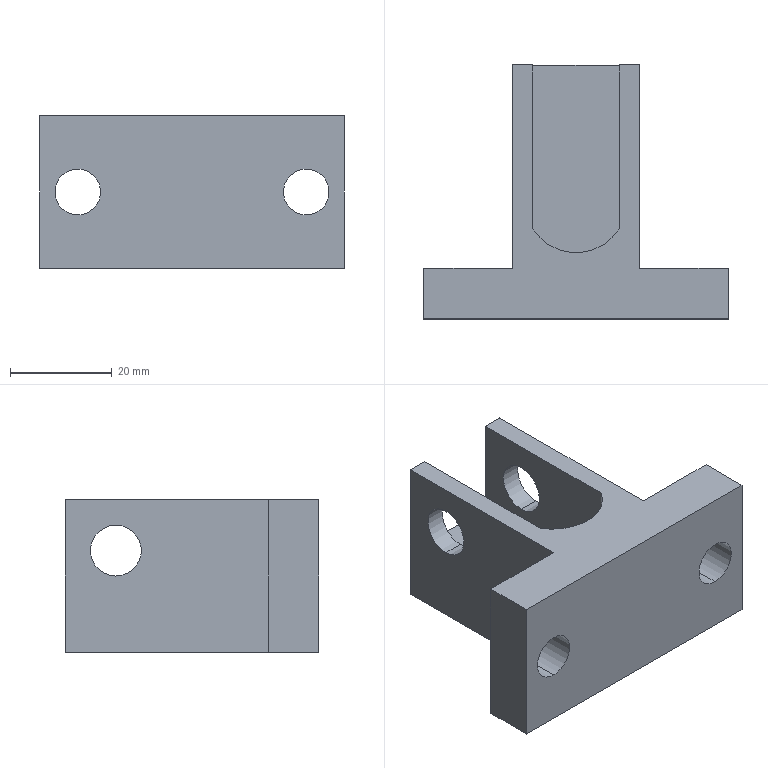Part | SolidWorks | features BaseBody 1 | 1 solid | 22 faces | box 60 x 50 x 30 mm | volume 33992 mm3 | plane 13 | cylinder 9 | commonest cylinder face diameters 9 x4 10 x4 20 x1
STEP:
#1=CARTESIAN_POINT('',(52.5,10.,19.5));
#2=VERTEX_POINT('',#1);
#3=CARTESIAN_POINT('',(52.5,10.,10.5));
#4=VERTEX_POINT('',#3);
#5=CARTESIAN_POINT('',(52.5,10.,15.));
#6=DIRECTION('',(0.,-1.,0.));
#7=DIRECTION('',(0.,0.,-1.));
#8=AXIS2_PLACEMENT_3D('',#5,#6,#7);
#9=CIRCLE('',#8,4.5);
#10=EDGE_CURVE('',#2,#4,#9,.T.);
#11=ORIENTED_EDGE('',*,*,#10,.F.);
#12=CARTESIAN_POINT('',(52.5,0.,19.5));
#13=VERTEX_POINT('',#12);
#14=CARTESIAN_POINT('',(52.5,0.,19.5));
#15=DIRECTION('',(0.,-1.,0.));
#16=VECTOR('',#15,1000.);
#17=LINE('',#14,#16);
#18=EDGE_CURVE('',#2,#13,#17,.T.);
#19=ORIENTED_EDGE('',*,*,#18,.T.);
#20=CARTESIAN_POINT('',(52.5,0.,10.5));
#21=VERTEX_POINT('',#20);
#22=CARTESIAN_POINT('',(52.5,0.,15.));
#23=DIRECTION('',(0.,-1.,0.));
#24=DIRECTION('',(0.,0.,-1.));
#25=AXIS2_PLACEMENT_3D('',#22,#23,#24);
#26=CIRCLE('',#25,4.5);
#27=EDGE_CURVE('',#13,#21,#26,.T.);
#28=ORIENTED_EDGE('',*,*,#27,.T.);
#29=CARTESIAN_POINT('',(52.5,0.,10.5));
#30=DIRECTION('',(0.,-1.,0.));
#31=VECTOR('',#30,1000.);
#32=LINE('',#29,#31);
#33=EDGE_CURVE('',#4,#21,#32,.T.);
#34=ORIENTED_EDGE('',*,*,#33,.F.);
#35=EDGE_LOOP('',(#11,#19,#28,#34));
#36=FACE_OUTER_BOUND('',#35,.T.);
#37=CARTESIAN_POINT('',(52.5,0.,15.));
#38=DIRECTION('',(0.,-1.,0.));
#39=DIRECTION('',(0.,0.,-1.));
#40=AXIS2_PLACEMENT_3D('',#37,#38,#39);
#41=CYLINDRICAL_SURFACE('',#40,4.5);
#42=ADVANCED_FACE('',(#36),#41,.F.);
#43=CARTESIAN_POINT('',(7.5,10.,19.5));
#44=VERTEX_POINT('',#43);
#45=CARTESIAN_POINT('',(7.5,10.,10.5));
#46=VERTEX_POINT('',#45);
#47=CARTESIAN_POINT('',(7.5,10.,15.));
#48=DIRECTION('',(0.,-1.,0.));
#49=DIRECTION('',(0.,0.,-1.));
#50=AXIS2_PLACEMENT_3D('',#47,#48,#49);
#51=CIRCLE('',#50,4.5);
#52=EDGE_CURVE('',#44,#46,#51,.T.);
#53=ORIENTED_EDGE('',*,*,#52,.F.);
#54=CARTESIAN_POINT('',(7.5,0.,19.5));
#55=VERTEX_POINT('',#54);
#56=CARTESIAN_POINT('',(7.5,0.,19.5));
#57=DIRECTION('',(0.,-1.,0.));
#58=VECTOR('',#57,1000.);
#59=LINE('',#56,#58);
#60=EDGE_CURVE('',#44,#55,#59,.T.);
#61=ORIENTED_EDGE('',*,*,#60,.T.);
#62=CARTESIAN_POINT('',(7.5,0.,10.5));
#63=VERTEX_POINT('',#62);
#64=CARTESIAN_POINT('',(7.5,0.,15.));
#65=DIRECTION('',(0.,-1.,0.));
#66=DIRECTION('',(0.,0.,-1.));
#67=AXIS2_PLACEMENT_3D('',#64,#65,#66);
#68=CIRCLE('',#67,4.5);
#69=EDGE_CURVE('',#55,#63,#68,.T.);
#70=ORIENTED_EDGE('',*,*,#69,.T.);
#71=CARTESIAN_POINT('',(7.5,0.,10.5));
#72=DIRECTION('',(0.,-1.,0.));
#73=VECTOR('',#72,1000.);
#74=LINE('',#71,#73);
#75=EDGE_CURVE('',#46,#63,#74,.T.);
#76=ORIENTED_EDGE('',*,*,#75,.F.);
#77=EDGE_LOOP('',(#53,#61,#70,#76));
#78=FACE_OUTER_BOUND('',#77,.T.);
#79=CARTESIAN_POINT('',(7.5,0.,15.));
#80=DIRECTION('',(0.,-1.,0.));
#81=DIRECTION('',(0.,0.,-1.));
#82=AXIS2_PLACEMENT_3D('',#79,#80,#81);
#83=CYLINDRICAL_SURFACE('',#82,4.5);
#84=ADVANCED_FACE('',(#78),#83,.F.);
#85=CARTESIAN_POINT('',(42.5,40.,25.));
#86=VERTEX_POINT('',#85);
#87=CARTESIAN_POINT('',(42.5,40.,15.));
#88=VERTEX_POINT('',#87);
#89=CARTESIAN_POINT('',(42.5,40.,20.));
#90=DIRECTION('',(1.,0.,0.));
#91=DIRECTION('',(0.,0.,1.));
#92=AXIS2_PLACEMENT_3D('',#89,#90,#91);
#93=CIRCLE('',#92,5.);
#94=EDGE_CURVE('',#86,#88,#93,.T.);
#95=ORIENTED_EDGE('',*,*,#94,.T.);
#96=CARTESIAN_POINT('',(38.5,40.,15.));
#97=VERTEX_POINT('',#96);
#98=CARTESIAN_POINT('',(60.,40.,15.));
#99=DIRECTION('',(-1.,0.,0.));
#100=VECTOR('',#99,1000.);
#101=LINE('',#98,#100);
#102=EDGE_CURVE('',#88,#97,#101,.T.);
#103=ORIENTED_EDGE('',*,*,#102,.T.);
#104=CARTESIAN_POINT('',(38.5,40.,25.));
#105=VERTEX_POINT('',#104);
#106=CARTESIAN_POINT('',(38.5,40.,20.));
#107=DIRECTION('',(-1.,0.,0.));
#108=DIRECTION('',(0.,0.,1.));
#109=AXIS2_PLACEMENT_3D('',#106,#107,#108);
#110=CIRCLE('',#109,5.);
#111=EDGE_CURVE('',#97,#105,#110,.T.);
#112=ORIENTED_EDGE('',*,*,#111,.T.);
#113=CARTESIAN_POINT('',(60.,40.,25.));
#114=DIRECTION('',(-1.,0.,0.));
#115=VECTOR('',#114,1000.);
#116=LINE('',#113,#115);
#117=EDGE_CURVE('',#86,#105,#116,.T.);
#118=ORIENTED_EDGE('',*,*,#117,.F.);
#119=EDGE_LOOP('',(#95,#103,#112,#118));
#120=FACE_OUTER_BOUND('',#119,.T.);
#121=CARTESIAN_POINT('',(60.,40.,20.));
#122=DIRECTION('',(-1.,0.,0.));
#123=DIRECTION('',(0.,0.,1.));
#124=AXIS2_PLACEMENT_3D('',#121,#122,#123);
#125=CYLINDRICAL_SURFACE('',#124,5.);
#126=ADVANCED_FACE('',(#120),#125,.F.);
#127=CARTESIAN_POINT('',(21.5,40.,25.));
#128=VERTEX_POINT('',#127);
#129=CARTESIAN_POINT('',(21.5,40.,15.));
#130=VERTEX_POINT('',#129);
#131=CARTESIAN_POINT('',(21.5,40.,20.));
#132=DIRECTION('',(1.,0.,0.));
#133=DIRECTION('',(0.,0.,1.));
#134=AXIS2_PLACEMENT_3D('',#131,#132,#133);
#135=CIRCLE('',#134,5.);
#136=EDGE_CURVE('',#128,#130,#135,.T.);
#137=ORIENTED_EDGE('',*,*,#136,.T.);
#138=CARTESIAN_POINT('',(17.5,40.,15.));
#139=VERTEX_POINT('',#138);
#140=CARTESIAN_POINT('',(60.,40.,15.));
#141=DIRECTION('',(-1.,0.,0.));
#142=VECTOR('',#141,1000.);
#143=LINE('',#140,#142);
#144=EDGE_CURVE('',#130,#139,#143,.T.);
#145=ORIENTED_EDGE('',*,*,#144,.T.);
#146=CARTESIAN_POINT('',(17.5,40.,25.));
#147=VERTEX_POINT('',#146);
#148=CARTESIAN_POINT('',(17.5,40.,20.));
#149=DIRECTION('',(-1.,0.,0.));
#150=DIRECTION('',(0.,0.,1.));
#151=AXIS2_PLACEMENT_3D('',#148,#149,#150);
#152=CIRCLE('',#151,5.);
#153=EDGE_CURVE('',#139,#147,#152,.T.);
#154=ORIENTED_EDGE('',*,*,#153,.T.);
#155=CARTESIAN_POINT('',(60.,40.,25.));
#156=DIRECTION('',(-1.,0.,0.));
#157=VECTOR('',#156,1000.);
#158=LINE('',#155,#157);
#159=EDGE_CURVE('',#128,#147,#158,.T.);
#160=ORIENTED_EDGE('',*,*,#159,.F.);
#161=EDGE_LOOP('',(#137,#145,#154,#160));
#162=FACE_OUTER_BOUND('',#161,.T.);
#163=CARTESIAN_POINT('',(60.,40.,20.));
#164=DIRECTION('',(-1.,0.,0.));
#165=DIRECTION('',(0.,0.,1.));
#166=AXIS2_PLACEMENT_3D('',#163,#164,#165);
#167=CYLINDRICAL_SURFACE('',#166,5.);
#168=ADVANCED_FACE('',(#162),#167,.F.);
#169=CARTESIAN_POINT('',(60.,0.,30.));
#170=VERTEX_POINT('',#169);
#171=CARTESIAN_POINT('',(60.,0.,0.));
#172=VERTEX_POINT('',#171);
#173=CARTESIAN_POINT('',(60.,0.,30.));
#174=DIRECTION('',(0.,0.,-1.));
#175=VECTOR('',#174,1000.);
#176=LINE('',#173,#175);
#177=EDGE_CURVE('',#170,#172,#176,.T.);
#178=ORIENTED_EDGE('',*,*,#177,.F.);
#179=CARTESIAN_POINT('',(0.,0.,30.));
#180=VERTEX_POINT('',#179);
#181=CARTESIAN_POINT('',(60.,0.,30.));
#182=DIRECTION('',(1.,0.,0.));
#183=VECTOR('',#182,1000.);
#184=LINE('',#181,#183);
#185=EDGE_CURVE('',#180,#170,#184,.T.);
#186=ORIENTED_EDGE('',*,*,#185,.F.);
#187=CARTESIAN_POINT('',(0.,0.,0.));
#188=VERTEX_POINT('',#187);
#189=CARTESIAN_POINT('',(0.,0.,30.));
#190=DIRECTION('',(0.,0.,1.));
#191=VECTOR('',#190,1000.);
#192=LINE('',#189,#191);
#193=EDGE_CURVE('',#188,#180,#192,.T.);
#194=ORIENTED_EDGE('',*,*,#193,.F.);
#195=CARTESIAN_POINT('',(60.,0.,0.));
#196=DIRECTION('',(-1.,0.,0.));
#197=VECTOR('',#196,1000.);
#198=LINE('',#195,#197);
#199=EDGE_CURVE('',#172,#188,#198,.T.);
#200=ORIENTED_EDGE('',*,*,#199,.F.);
#201=EDGE_LOOP('',(#178,#186,#194,#200));
#202=FACE_OUTER_BOUND('',#201,.T.);
#203=CARTESIAN_POINT('',(52.5,0.,15.));
#204=DIRECTION('',(0.,-1.,0.));
#205=DIRECTION('',(0.,0.,-1.));
#206=AXIS2_PLACEMENT_3D('',#203,#204,#205);
#207=CIRCLE('',#206,4.5);
#208=EDGE_CURVE('',#21,#13,#207,.T.);
#209=ORIENTED_EDGE('',*,*,#208,.F.);
#210=ORIENTED_EDGE('',*,*,#27,.F.);
#211=EDGE_LOOP('',(#209,#210));
#212=FACE_BOUND('',#211,.T.);
#213=CARTESIAN_POINT('',(7.5,0.,15.));
#214=DIRECTION('',(0.,-1.,0.));
#215=DIRECTION('',(0.,0.,-1.));
#216=AXIS2_PLACEMENT_3D('',#213,#214,#215);
#217=CIRCLE('',#216,4.5);
#218=EDGE_CURVE('',#63,#55,#217,.T.);
#219=ORIENTED_EDGE('',*,*,#218,.F.);
#220=ORIENTED_EDGE('',*,*,#69,.F.);
#221=EDGE_LOOP('',(#219,#220));
#222=FACE_BOUND('',#221,.T.);
#223=CARTESIAN_POINT('',(60.,0.,30.));
#224=DIRECTION('',(0.,1.,0.));
#225=DIRECTION('',(-1.,0.,0.));
#226=AXIS2_PLACEMENT_3D('',#223,#224,#225);
#227=PLANE('',#226);
#228=ADVANCED_FACE('',(#202,#212,#222),#227,.F.);
#229=CARTESIAN_POINT('',(42.5,10.,0.));
#230=VERTEX_POINT('',#229);
#231=CARTESIAN_POINT('',(60.,10.,0.));
#232=VERTEX_POINT('',#231);
#233=CARTESIAN_POINT('',(0.,10.,0.));
#234=DIRECTION('',(1.,0.,0.));
#235=VECTOR('',#234,1000.);
#236=LINE('',#233,#235);
#237=EDGE_CURVE('',#230,#232,#236,.T.);
#238=ORIENTED_EDGE('',*,*,#237,.T.);
#239=CARTESIAN_POINT('',(60.,0.,0.));
#240=DIRECTION('',(0.,-1.,0.));
#241=VECTOR('',#240,1000.);
#242=LINE('',#239,#241);
#243=EDGE_CURVE('',#232,#172,#242,.T.);
#244=ORIENTED_EDGE('',*,*,#243,.T.);
#245=ORIENTED_EDGE('',*,*,#199,.T.);
#246=CARTESIAN_POINT('',(0.,10.,0.));
#247=VERTEX_POINT('',#246);
#248=CARTESIAN_POINT('',(0.,0.,0.));
#249=DIRECTION('',(0.,1.,0.));
#250=VECTOR('',#249,1000.);
#251=LINE('',#248,#250);
#252=EDGE_CURVE('',#188,#247,#251,.T.);
#253=ORIENTED_EDGE('',*,*,#252,.T.);
#254=CARTESIAN_POINT('',(17.5,10.,0.));
#255=VERTEX_POINT('',#254);
#256=CARTESIAN_POINT('',(0.,10.,0.));
#257=DIRECTION('',(1.,0.,0.));
#258=VECTOR('',#257,1000.);
#259=LINE('',#256,#258);
#260=EDGE_CURVE('',#247,#255,#259,.T.);
#261=ORIENTED_EDGE('',*,*,#260,.T.);
#262=CARTESIAN_POINT('',(17.5,50.,0.));
#263=VERTEX_POINT('',#262);
#264=CARTESIAN_POINT('',(17.5,0.,0.));
#265=DIRECTION('',(0.,1.,0.));
#266=VECTOR('',#265,1000.);
#267=LINE('',#264,#266);
#268=EDGE_CURVE('',#255,#263,#267,.T.);
#269=ORIENTED_EDGE('',*,*,#268,.T.);
#270=CARTESIAN_POINT('',(42.5,50.,0.));
#271=VERTEX_POINT('',#270);
#272=CARTESIAN_POINT('',(0.,50.,0.));
#273=DIRECTION('',(1.,0.,0.));
#274=VECTOR('',#273,1000.);
#275=LINE('',#272,#274);
#276=EDGE_CURVE('',#263,#271,#275,.T.);
#277=ORIENTED_EDGE('',*,*,#276,.T.);
#278=CARTESIAN_POINT('',(42.5,0.,0.));
#279=DIRECTION('',(0.,-1.,0.));
#280=VECTOR('',#279,1000.);
#281=LINE('',#278,#280);
#282=EDGE_CURVE('',#271,#230,#281,.T.);
#283=ORIENTED_EDGE('',*,*,#282,.T.);
#284=EDGE_LOOP('',(#238,#244,#245,#253,#261,#269,#277,#283));
#285=FACE_OUTER_BOUND('',#284,.T.);
#286=CARTESIAN_POINT('',(0.,0.,0.));
#287=DIRECTION('',(0.,0.,-1.));
#288=DIRECTION('',(-1.,0.,0.));
#289=AXIS2_PLACEMENT_3D('',#286,#287,#288);
#290=PLANE('',#289);
#291=ADVANCED_FACE('',(#285),#290,.T.);
#292=CARTESIAN_POINT('',(60.,10.,30.));
#293=VERTEX_POINT('',#292);
#294=CARTESIAN_POINT('',(60.,10.,30.));
#295=DIRECTION('',(0.,0.,-1.));
#296=VECTOR('',#295,1000.);
#297=LINE('',#294,#296);
#298=EDGE_CURVE('',#293,#232,#297,.T.);
#299=ORIENTED_EDGE('',*,*,#298,.F.);
#300=CARTESIAN_POINT('',(60.,10.,30.));
#301=DIRECTION('',(0.,1.,0.));
#302=VECTOR('',#301,1000.);
#303=LINE('',#300,#302);
#304=EDGE_CURVE('',#170,#293,#303,.T.);
#305=ORIENTED_EDGE('',*,*,#304,.F.);
#306=ORIENTED_EDGE('',*,*,#177,.T.);
#307=ORIENTED_EDGE('',*,*,#243,.F.);
#308=EDGE_LOOP('',(#299,#305,#306,#307));
#309=FACE_OUTER_BOUND('',#308,.T.);
#310=CARTESIAN_POINT('',(60.,10.,30.));
#311=DIRECTION('',(-1.,0.,0.));
#312=DIRECTION('',(0.,0.,1.));
#313=AXIS2_PLACEMENT_3D('',#310,#311,#312);
#314=PLANE('',#313);
#315=ADVANCED_FACE('',(#309),#314,.F.);
#316=CARTESIAN_POINT('',(38.5,17.732,30.));
#317=VERTEX_POINT('',#316);
#318=CARTESIAN_POINT('',(38.5,50.,30.));
#319=VERTEX_POINT('',#318);
#320=CARTESIAN_POINT('',(38.5,0.,30.));
#321=DIRECTION('',(0.,1.,0.));
#322=VECTOR('',#321,1000.);
#323=LINE('',#320,#322);
#324=EDGE_CURVE('',#317,#319,#323,.T.);
#325=ORIENTED_EDGE('',*,*,#324,.F.);
#326=CARTESIAN_POINT('',(21.5,17.732,30.));
#327=VERTEX_POINT('',#326);
#328=CARTESIAN_POINT('',(30.,23.,30.));
#329=DIRECTION('',(0.,0.,1.));
#330=DIRECTION('',(1.,0.,0.));
#331=AXIS2_PLACEMENT_3D('',#328,#329,#330);
#332=CIRCLE('',#331,10.);
#333=EDGE_CURVE('',#327,#317,#332,.T.);
#334=ORIENTED_EDGE('',*,*,#333,.F.);
#335=CARTESIAN_POINT('',(21.5,50.,30.));
#336=VERTEX_POINT('',#335);
#337=CARTESIAN_POINT('',(21.5,0.,30.));
#338=DIRECTION('',(0.,-1.,0.));
#339=VECTOR('',#338,1000.);
#340=LINE('',#337,#339);
#341=EDGE_CURVE('',#336,#327,#340,.T.);
#342=ORIENTED_EDGE('',*,*,#341,.F.);
#343=CARTESIAN_POINT('',(17.5,50.,30.));
#344=VERTEX_POINT('',#343);
#345=CARTESIAN_POINT('',(0.,50.,30.));
#346=DIRECTION('',(1.,0.,0.));
#347=VECTOR('',#346,1000.);
#348=LINE('',#345,#347);
#349=EDGE_CURVE('',#344,#336,#348,.T.);
#350=ORIENTED_EDGE('',*,*,#349,.F.);
#351=CARTESIAN_POINT('',(17.5,10.,30.));
#352=VERTEX_POINT('',#351);
#353=CARTESIAN_POINT('',(17.5,0.,30.));
#354=DIRECTION('',(0.,1.,0.));
#355=VECTOR('',#354,1000.);
#356=LINE('',#353,#355);
#357=EDGE_CURVE('',#352,#344,#356,.T.);
#358=ORIENTED_EDGE('',*,*,#357,.F.);
#359=CARTESIAN_POINT('',(0.,10.,30.));
#360=VERTEX_POINT('',#359);
#361=CARTESIAN_POINT('',(0.,10.,30.));
#362=DIRECTION('',(1.,0.,0.));
#363=VECTOR('',#362,1000.);
#364=LINE('',#361,#363);
#365=EDGE_CURVE('',#360,#352,#364,.T.);
#366=ORIENTED_EDGE('',*,*,#365,.F.);
#367=CARTESIAN_POINT('',(0.,0.,30.));
#368=DIRECTION('',(0.,1.,0.));
#369=VECTOR('',#368,1000.);
#370=LINE('',#367,#369);
#371=EDGE_CURVE('',#180,#360,#370,.T.);
#372=ORIENTED_EDGE('',*,*,#371,.F.);
#373=ORIENTED_EDGE('',*,*,#185,.T.);
#374=ORIENTED_EDGE('',*,*,#304,.T.);
#375=CARTESIAN_POINT('',(42.5,10.,30.));
#376=VERTEX_POINT('',#375);
#377=CARTESIAN_POINT('',(0.,10.,30.));
#378=DIRECTION('',(1.,0.,0.));
#379=VECTOR('',#378,1000.);
#380=LINE('',#377,#379);
#381=EDGE_CURVE('',#376,#293,#380,.T.);
#382=ORIENTED_EDGE('',*,*,#381,.F.);
#383=CARTESIAN_POINT('',(42.5,50.,30.));
#384=VERTEX_POINT('',#383);
#385=CARTESIAN_POINT('',(42.5,0.,30.));
#386=DIRECTION('',(0.,-1.,0.));
#387=VECTOR('',#386,1000.);
#388=LINE('',#385,#387);
#389=EDGE_CURVE('',#384,#376,#388,.T.);
#390=ORIENTED_EDGE('',*,*,#389,.F.);
#391=CARTESIAN_POINT('',(0.,50.,30.));
#392=DIRECTION('',(1.,0.,0.));
#393=VECTOR('',#392,1000.);
#394=LINE('',#391,#393);
#395=EDGE_CURVE('',#319,#384,#394,.T.);
#396=ORIENTED_EDGE('',*,*,#395,.F.);
#397=EDGE_LOOP('',(#325,#334,#342,#350,#358,#366,#372,#373,#374,#382,#390,#396));
#398=FACE_OUTER_BOUND('',#397,.T.);
#399=CARTESIAN_POINT('',(0.,0.,30.));
#400=DIRECTION('',(0.,0.,-1.));
#401=DIRECTION('',(-1.,0.,0.));
#402=AXIS2_PLACEMENT_3D('',#399,#400,#401);
#403=PLANE('',#402);
#404=ADVANCED_FACE('',(#398),#403,.F.);
#405=ORIENTED_EDGE('',*,*,#193,.T.);
#406=ORIENTED_EDGE('',*,*,#371,.T.);
#407=CARTESIAN_POINT('',(0.,10.,30.));
#408=DIRECTION('',(0.,0.,1.));
#409=VECTOR('',#408,1000.);
#410=LINE('',#407,#409);
#411=EDGE_CURVE('',#247,#360,#410,.T.);
#412=ORIENTED_EDGE('',*,*,#411,.F.);
#413=ORIENTED_EDGE('',*,*,#252,.F.);
#414=EDGE_LOOP('',(#405,#406,#412,#413));
#415=FACE_OUTER_BOUND('',#414,.T.);
#416=CARTESIAN_POINT('',(0.,0.,30.));
#417=DIRECTION('',(1.,0.,0.));
#418=DIRECTION('',(0.,0.,-1.));
#419=AXIS2_PLACEMENT_3D('',#416,#417,#418);
#420=PLANE('',#419);
#421=ADVANCED_FACE('',(#415),#420,.F.);
#422=ORIENTED_EDGE('',*,*,#18,.F.);
#423=CARTESIAN_POINT('',(52.5,10.,15.));
#424=DIRECTION('',(0.,-1.,0.));
#425=DIRECTION('',(0.,0.,-1.));
#426=AXIS2_PLACEMENT_3D('',#423,#424,#425);
#427=CIRCLE('',#426,4.5);
#428=EDGE_CURVE('',#4,#2,#427,.T.);
#429=ORIENTED_EDGE('',*,*,#428,.F.);
#430=ORIENTED_EDGE('',*,*,#33,.T.);
#431=ORIENTED_EDGE('',*,*,#208,.T.);
#432=EDGE_LOOP('',(#422,#429,#430,#431));
#433=FACE_OUTER_BOUND('',#432,.T.);
#434=CARTESIAN_POINT('',(52.5,0.,15.));
#435=DIRECTION('',(0.,-1.,0.));
#436=DIRECTION('',(0.,0.,-1.));
#437=AXIS2_PLACEMENT_3D('',#434,#435,#436);
#438=CYLINDRICAL_SURFACE('',#437,4.5);
#439=ADVANCED_FACE('',(#433),#438,.F.);
#440=ORIENTED_EDGE('',*,*,#60,.F.);
#441=CARTESIAN_POINT('',(7.5,10.,15.));
#442=DIRECTION('',(0.,-1.,0.));
#443=DIRECTION('',(0.,0.,-1.));
#444=AXIS2_PLACEMENT_3D('',#441,#442,#443);
#445=CIRCLE('',#444,4.5);
#446=EDGE_CURVE('',#46,#44,#445,.T.);
#447=ORIENTED_EDGE('',*,*,#446,.F.);
#448=ORIENTED_EDGE('',*,*,#75,.T.);
#449=ORIENTED_EDGE('',*,*,#218,.T.);
#450=EDGE_LOOP('',(#440,#447,#448,#449));
#451=FACE_OUTER_BOUND('',#450,.T.);
#452=CARTESIAN_POINT('',(7.5,0.,15.));
#453=DIRECTION('',(0.,-1.,0.));
#454=DIRECTION('',(0.,0.,-1.));
#455=AXIS2_PLACEMENT_3D('',#452,#453,#454);
#456=CYLINDRICAL_SURFACE('',#455,4.5);
#457=ADVANCED_FACE('',(#451),#456,.F.);
#458=CARTESIAN_POINT('',(42.5,10.,30.));
#459=DIRECTION('',(0.,0.,-1.));
#460=VECTOR('',#459,1000.);
#461=LINE('',#458,#460);
#462=EDGE_CURVE('',#376,#230,#461,.T.);
#463=ORIENTED_EDGE('',*,*,#462,.F.);
#464=ORIENTED_EDGE('',*,*,#381,.T.);
#465=ORIENTED_EDGE('',*,*,#298,.T.);
#466=ORIENTED_EDGE('',*,*,#237,.F.);
#467=EDGE_LOOP('',(#463,#464,#465,#466));
#468=FACE_OUTER_BOUND('',#467,.T.);
#469=ORIENTED_EDGE('',*,*,#428,.T.);
#470=ORIENTED_EDGE('',*,*,#10,.T.);
#471=EDGE_LOOP('',(#469,#470));
#472=FACE_BOUND('',#471,.T.);
#473=CARTESIAN_POINT('',(42.5,10.,30.));
#474=DIRECTION('',(0.,-1.,0.));
#475=DIRECTION('',(0.,0.,-1.));
#476=AXIS2_PLACEMENT_3D('',#473,#474,#475);
#477=PLANE('',#476);
#478=ADVANCED_FACE('',(#468,#472),#477,.F.);
#479=CARTESIAN_POINT('',(42.5,50.,30.));
#480=DIRECTION('',(0.,0.,-1.));
#481=VECTOR('',#480,1000.);
#482=LINE('',#479,#481);
#483=EDGE_CURVE('',#384,#271,#482,.T.);
#484=ORIENTED_EDGE('',*,*,#483,.F.);
#485=ORIENTED_EDGE('',*,*,#389,.T.);
#486=ORIENTED_EDGE('',*,*,#462,.T.);
#487=ORIENTED_EDGE('',*,*,#282,.F.);
#488=EDGE_LOOP('',(#484,#485,#486,#487));
#489=FACE_OUTER_BOUND('',#488,.T.);
#490=ORIENTED_EDGE('',*,*,#94,.F.);
#491=CARTESIAN_POINT('',(42.5,40.,20.));
#492=DIRECTION('',(1.,0.,0.));
#493=DIRECTION('',(0.,0.,1.));
#494=AXIS2_PLACEMENT_3D('',#491,#492,#493);
#495=CIRCLE('',#494,5.);
#496=EDGE_CURVE('',#88,#86,#495,.T.);
#497=ORIENTED_EDGE('',*,*,#496,.F.);
#498=EDGE_LOOP('',(#490,#497));
#499=FACE_BOUND('',#498,.T.);
#500=CARTESIAN_POINT('',(42.5,50.,30.));
#501=DIRECTION('',(-1.,0.,0.));
#502=DIRECTION('',(0.,0.,1.));
#503=AXIS2_PLACEMENT_3D('',#500,#501,#502);
#504=PLANE('',#503);
#505=ADVANCED_FACE('',(#489,#499),#504,.F.);
#506=CARTESIAN_POINT('',(38.5,50.,10.));
#507=VERTEX_POINT('',#506);
#508=CARTESIAN_POINT('',(38.5,50.,30.));
#509=DIRECTION('',(0.,0.,-1.));
#510=VECTOR('',#509,1000.);
#511=LINE('',#508,#510);
#512=EDGE_CURVE('',#319,#507,#511,.T.);
#513=ORIENTED_EDGE('',*,*,#512,.F.);
#514=ORIENTED_EDGE('',*,*,#395,.T.);
#515=ORIENTED_EDGE('',*,*,#483,.T.);
#516=ORIENTED_EDGE('',*,*,#276,.F.);
#517=CARTESIAN_POINT('',(17.5,50.,30.));
#518=DIRECTION('',(0.,0.,-1.));
#519=VECTOR('',#518,1000.);
#520=LINE('',#517,#519);
#521=EDGE_CURVE('',#344,#263,#520,.T.);
#522=ORIENTED_EDGE('',*,*,#521,.F.);
#523=ORIENTED_EDGE('',*,*,#349,.T.);
#524=CARTESIAN_POINT('',(21.5,50.,10.));
#525=VERTEX_POINT('',#524);
#526=CARTESIAN_POINT('',(21.5,50.,30.));
#527=DIRECTION('',(0.,0.,1.));
#528=VECTOR('',#527,1000.);
#529=LINE('',#526,#528);
#530=EDGE_CURVE('',#525,#336,#529,.T.);
#531=ORIENTED_EDGE('',*,*,#530,.F.);
#532=CARTESIAN_POINT('',(17.5,50.,10.));
#533=DIRECTION('',(-1.,0.,0.));
#534=VECTOR('',#533,1000.);
#535=LINE('',#532,#534);
#536=EDGE_CURVE('',#507,#525,#535,.T.);
#537=ORIENTED_EDGE('',*,*,#536,.F.);
#538=EDGE_LOOP('',(#513,#514,#515,#516,#522,#523,#531,#537));
#539=FACE_OUTER_BOUND('',#538,.T.);
#540=CARTESIAN_POINT('',(17.5,50.,30.));
#541=DIRECTION('',(0.,-1.,0.));
#542=DIRECTION('',(0.,0.,-1.));
#543=AXIS2_PLACEMENT_3D('',#540,#541,#542);
#544=PLANE('',#543);
#545=ADVANCED_FACE('',(#539),#544,.F.);
#546=CARTESIAN_POINT('',(17.5,10.,30.));
#547=DIRECTION('',(0.,0.,-1.));
#548=VECTOR('',#547,1000.);
#549=LINE('',#546,#548);
#550=EDGE_CURVE('',#352,#255,#549,.T.);
#551=ORIENTED_EDGE('',*,*,#550,.F.);
#552=ORIENTED_EDGE('',*,*,#357,.T.);
#553=ORIENTED_EDGE('',*,*,#521,.T.);
#554=ORIENTED_EDGE('',*,*,#268,.F.);
#555=EDGE_LOOP('',(#551,#552,#553,#554));
#556=FACE_OUTER_BOUND('',#555,.T.);
#557=CARTESIAN_POINT('',(17.5,40.,20.));
#558=DIRECTION('',(-1.,0.,0.));
#559=DIRECTION('',(0.,0.,1.));
#560=AXIS2_PLACEMENT_3D('',#557,#558,#559);
#561=CIRCLE('',#560,5.);
#562=EDGE_CURVE('',#147,#139,#561,.T.);
#563=ORIENTED_EDGE('',*,*,#562,.F.);
#564=ORIENTED_EDGE('',*,*,#153,.F.);
#565=EDGE_LOOP('',(#563,#564));
#566=FACE_BOUND('',#565,.T.);
#567=CARTESIAN_POINT('',(17.5,10.,30.));
#568=DIRECTION('',(1.,0.,0.));
#569=DIRECTION('',(0.,0.,-1.));
#570=AXIS2_PLACEMENT_3D('',#567,#568,#569);
#571=PLANE('',#570);
#572=ADVANCED_FACE('',(#556,#566),#571,.F.);
#573=ORIENTED_EDGE('',*,*,#411,.T.);
#574=ORIENTED_EDGE('',*,*,#365,.T.);
#575=ORIENTED_EDGE('',*,*,#550,.T.);
#576=ORIENTED_EDGE('',*,*,#260,.F.);
#577=EDGE_LOOP('',(#573,#574,#575,#576));
#578=FACE_OUTER_BOUND('',#577,.T.);
#579=ORIENTED_EDGE('',*,*,#446,.T.);
#580=ORIENTED_EDGE('',*,*,#52,.T.);
#581=EDGE_LOOP('',(#579,#580));
#582=FACE_BOUND('',#581,.T.);
#583=CARTESIAN_POINT('',(0.,10.,30.));
#584=DIRECTION('',(0.,-1.,0.));
#585=DIRECTION('',(0.,0.,-1.));
#586=AXIS2_PLACEMENT_3D('',#583,#584,#585);
#587=PLANE('',#586);
#588=ADVANCED_FACE('',(#578,#582),#587,.F.);
#589=CARTESIAN_POINT('',(38.5,17.732,10.));
#590=VERTEX_POINT('',#589);
#591=CARTESIAN_POINT('',(38.5,17.732,10.));
#592=DIRECTION('',(0.,0.,-1.));
#593=VECTOR('',#592,1000.);
#594=LINE('',#591,#593);
#595=EDGE_CURVE('',#317,#590,#594,.T.);
#596=ORIENTED_EDGE('',*,*,#595,.F.);
#597=ORIENTED_EDGE('',*,*,#324,.T.);
#598=ORIENTED_EDGE('',*,*,#512,.T.);
#599=CARTESIAN_POINT('',(38.5,68.657,10.));
#600=DIRECTION('',(0.,1.,0.));
#601=VECTOR('',#600,1000.);
#602=LINE('',#599,#601);
#603=EDGE_CURVE('',#590,#507,#602,.T.);
#604=ORIENTED_EDGE('',*,*,#603,.F.);
#605=EDGE_LOOP('',(#596,#597,#598,#604));
#606=FACE_OUTER_BOUND('',#605,.T.);
#607=CARTESIAN_POINT('',(38.5,40.,20.));
#608=DIRECTION('',(-1.,0.,0.));
#609=DIRECTION('',(0.,0.,1.));
#610=AXIS2_PLACEMENT_3D('',#607,#608,#609);
#611=CIRCLE('',#610,5.);
#612=EDGE_CURVE('',#105,#97,#611,.T.);
#613=ORIENTED_EDGE('',*,*,#612,.F.);
#614=ORIENTED_EDGE('',*,*,#111,.F.);
#615=EDGE_LOOP('',(#613,#614));
#616=FACE_BOUND('',#615,.T.);
#617=CARTESIAN_POINT('',(38.5,68.657,10.));
#618=DIRECTION('',(1.,0.,0.));
#619=DIRECTION('',(0.,1.,0.));
#620=AXIS2_PLACEMENT_3D('',#617,#618,#619);
#621=PLANE('',#620);
#622=ADVANCED_FACE('',(#606,#616),#621,.F.);
#623=ORIENTED_EDGE('',*,*,#595,.T.);
#624=CARTESIAN_POINT('',(21.5,17.732,10.));
#625=VERTEX_POINT('',#624);
#626=CARTESIAN_POINT('',(30.,23.,10.));
#627=DIRECTION('',(0.,0.,1.));
#628=DIRECTION('',(1.,0.,0.));
#629=AXIS2_PLACEMENT_3D('',#626,#627,#628);
#630=CIRCLE('',#629,10.);
#631=EDGE_CURVE('',#625,#590,#630,.T.);
#632=ORIENTED_EDGE('',*,*,#631,.F.);
#633=CARTESIAN_POINT('',(21.5,17.732,10.));
#634=DIRECTION('',(0.,0.,-1.));
#635=VECTOR('',#634,1000.);
#636=LINE('',#633,#635);
#637=EDGE_CURVE('',#327,#625,#636,.T.);
#638=ORIENTED_EDGE('',*,*,#637,.F.);
#639=ORIENTED_EDGE('',*,*,#333,.T.);
#640=EDGE_LOOP('',(#623,#632,#638,#639));
#641=FACE_OUTER_BOUND('',#640,.T.);
#642=CARTESIAN_POINT('',(30.,23.,10.));
#643=DIRECTION('',(0.,0.,1.));
#644=DIRECTION('',(1.,0.,0.));
#645=AXIS2_PLACEMENT_3D('',#642,#643,#644);
#646=CYLINDRICAL_SURFACE('',#645,10.);
#647=ADVANCED_FACE('',(#641),#646,.F.);
#648=ORIENTED_EDGE('',*,*,#637,.T.);
#649=CARTESIAN_POINT('',(21.5,68.657,10.));
#650=DIRECTION('',(0.,-1.,0.));
#651=VECTOR('',#650,1000.);
#652=LINE('',#649,#651);
#653=EDGE_CURVE('',#525,#625,#652,.T.);
#654=ORIENTED_EDGE('',*,*,#653,.F.);
#655=ORIENTED_EDGE('',*,*,#530,.T.);
#656=ORIENTED_EDGE('',*,*,#341,.T.);
#657=EDGE_LOOP('',(#648,#654,#655,#656));
#658=FACE_OUTER_BOUND('',#657,.T.);
#659=ORIENTED_EDGE('',*,*,#136,.F.);
#660=CARTESIAN_POINT('',(21.5,40.,20.));
#661=DIRECTION('',(1.,0.,0.));
#662=DIRECTION('',(0.,0.,1.));
#663=AXIS2_PLACEMENT_3D('',#660,#661,#662);
#664=CIRCLE('',#663,5.);
#665=EDGE_CURVE('',#130,#128,#664,.T.);
#666=ORIENTED_EDGE('',*,*,#665,.F.);
#667=EDGE_LOOP('',(#659,#666));
#668=FACE_BOUND('',#667,.T.);
#669=CARTESIAN_POINT('',(21.5,68.657,10.));
#670=DIRECTION('',(-1.,0.,0.));
#671=DIRECTION('',(0.,-1.,0.));
#672=AXIS2_PLACEMENT_3D('',#669,#670,#671);
#673=PLANE('',#672);
#674=ADVANCED_FACE('',(#658,#668),#673,.F.);
#675=ORIENTED_EDGE('',*,*,#102,.F.);
#676=ORIENTED_EDGE('',*,*,#496,.T.);
#677=ORIENTED_EDGE('',*,*,#117,.T.);
#678=ORIENTED_EDGE('',*,*,#612,.T.);
#679=EDGE_LOOP('',(#675,#676,#677,#678));
#680=FACE_OUTER_BOUND('',#679,.T.);
#681=CARTESIAN_POINT('',(60.,40.,20.));
#682=DIRECTION('',(-1.,0.,0.));
#683=DIRECTION('',(0.,0.,1.));
#684=AXIS2_PLACEMENT_3D('',#681,#682,#683);
#685=CYLINDRICAL_SURFACE('',#684,5.);
#686=ADVANCED_FACE('',(#680),#685,.F.);
#687=ORIENTED_EDGE('',*,*,#631,.T.);
#688=ORIENTED_EDGE('',*,*,#603,.T.);
#689=ORIENTED_EDGE('',*,*,#536,.T.);
#690=ORIENTED_EDGE('',*,*,#653,.T.);
#691=EDGE_LOOP('',(#687,#688,#689,#690));
#692=FACE_OUTER_BOUND('',#691,.T.);
#693=CARTESIAN_POINT('',(30.,50.,10.));
#694=DIRECTION('',(0.,0.,1.));
#695=DIRECTION('',(1.,0.,0.));
#696=AXIS2_PLACEMENT_3D('',#693,#694,#695);
#697=PLANE('',#696);
#698=ADVANCED_FACE('',(#692),#697,.T.);
#699=ORIENTED_EDGE('',*,*,#144,.F.);
#700=ORIENTED_EDGE('',*,*,#665,.T.);
#701=ORIENTED_EDGE('',*,*,#159,.T.);
#702=ORIENTED_EDGE('',*,*,#562,.T.);
#703=EDGE_LOOP('',(#699,#700,#701,#702));
#704=FACE_OUTER_BOUND('',#703,.T.);
#705=CARTESIAN_POINT('',(60.,40.,20.));
#706=DIRECTION('',(-1.,0.,0.));
#707=DIRECTION('',(0.,0.,1.));
#708=AXIS2_PLACEMENT_3D('',#705,#706,#707);
#709=CYLINDRICAL_SURFACE('',#708,5.);
#710=ADVANCED_FACE('',(#704),#709,.F.);
#711=CLOSED_SHELL('',(#42,#84,#126,#168,#228,#291,#315,#404,#421,#439,#457,#478,#505,#545,#572,#588,#622,#647,#674,#686,#698,#710));
#712=MANIFOLD_SOLID_BREP('',#711);
#713=CARTESIAN_POINT('',(0.,0.,0.));
#714=DIRECTION('',(0.,0.,1.));
#715=DIRECTION('',(1.,0.,0.));
#716=AXIS2_PLACEMENT_3D('',#713,#714,#715);
#717=(LENGTH_UNIT()NAMED_UNIT(*)SI_UNIT(.MILLI.,.METRE.));
#718=UNCERTAINTY_MEASURE_WITH_UNIT(LENGTH_MEASURE(0.00001),#717,'','');
#719=(NAMED_UNIT(*)PLANE_ANGLE_UNIT()SI_UNIT($,.RADIAN.));
#720=(NAMED_UNIT(*)SI_UNIT($,.STERADIAN.)SOLID_ANGLE_UNIT());
#721=(GEOMETRIC_REPRESENTATION_CONTEXT(3)GLOBAL_UNCERTAINTY_ASSIGNED_CONTEXT((#718))GLOBAL_UNIT_ASSIGNED_CONTEXT((#717,#719,#720))REPRESENTATION_CONTEXT('',''));
#722=ADVANCED_BREP_SHAPE_REPRESENTATION('',(#712,#716),#721);